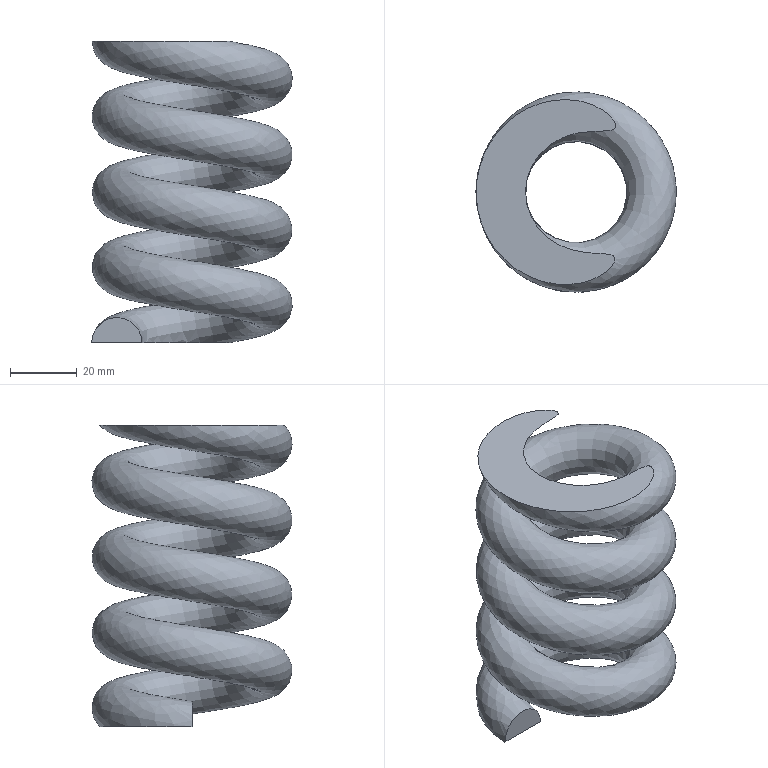Part | NX | features MAIN_BODY 2 | 1 solid | 4 faces | box 59.9 x 59.795 x 90 mm | volume 97193 mm3 | plane 3 | spline 1
STEP:
#1=CARTESIAN_POINT('',(-585.,25.,130.));
#2=VERTEX_POINT('',#1);
#3=CARTESIAN_POINT('',(-570.,25.,130.));
#4=VERTEX_POINT('',#3);
#5=CARTESIAN_POINT('',(-577.5,25.,130.));
#6=DIRECTION('',(0.,1.,0.));
#7=DIRECTION('',(0.,0.,-1.));
#8=AXIS2_PLACEMENT_3D('',#5,#6,#7);
#9=CIRCLE('',#8,7.5);
#10=EDGE_CURVE('',#2,#4,#9,.T.);
#11=ORIENTED_EDGE('',*,*,#10,.T.);
#12=CARTESIAN_POINT('',(-585.,25.,130.));
#13=CARTESIAN_POINT('',(-585.,27.045,130.));
#14=CARTESIAN_POINT('',(-584.488,31.04,130.));
#15=CARTESIAN_POINT('',(-581.859,38.786,130.));
#16=CARTESIAN_POINT('',(-576.924,45.368,130.));
#17=CARTESIAN_POINT('',(-570.139,49.94,130.));
#18=CARTESIAN_POINT('',(-564.47,52.09,130.));
#19=CARTESIAN_POINT('',(-559.395,52.727,130.));
#20=CARTESIAN_POINT('',(-555.366,52.475,130.));
#21=CARTESIAN_POINT('',(-552.35,51.874,130.));
#22=CARTESIAN_POINT('',(-549.498,50.852,130.));
#23=CARTESIAN_POINT('',(-547.249,49.607,130.));
#24=CARTESIAN_POINT('',(-545.63,48.346,130.));
#25=CARTESIAN_POINT('',(-544.556,47.258,130.));
#26=CARTESIAN_POINT('',(-543.829,46.178,130.));
#27=CARTESIAN_POINT('',(-543.527,45.186,130.));
#28=CARTESIAN_POINT('',(-543.63,44.385,130.));
#29=CARTESIAN_POINT('',(-544.226,43.836,130.));
#30=CARTESIAN_POINT('',(-545.199,43.494,130.));
#31=CARTESIAN_POINT('',(-546.469,43.349,130.));
#32=CARTESIAN_POINT('',(-548.002,43.281,130.));
#33=CARTESIAN_POINT('',(-550.045,43.207,130.));
#34=CARTESIAN_POINT('',(-552.6,43.018,130.));
#35=CARTESIAN_POINT('',(-555.61,42.46,130.));
#36=CARTESIAN_POINT('',(-558.514,41.525,130.));
#37=CARTESIAN_POINT('',(-562.2,39.726,130.));
#38=CARTESIAN_POINT('',(-566.15,36.439,130.));
#39=CARTESIAN_POINT('',(-569.39,31.132,130.));
#40=CARTESIAN_POINT('',(-570.,27.054,130.));
#41=CARTESIAN_POINT('',(-570.,25.,130.));
#42=B_SPLINE_CURVE_WITH_KNOTS('',3,(#12,#13,#14,#15,#16,#17,#18,#19,#20,#21,#22,#23,#24,#25,#26,#27,#28,#29,#30,#31,#32,#33,#34,#35,#36,#37,#38,#39,#40,#41),.UNSPECIFIED.,.F.,.F.,(4,1,1,1,1,1,1,1,1,1,1,1,1,1,1,1,1,1,1,1,1,1,1,1,1,1,1,4),(0.,0.006042,0.01208,0.02417,0.03021,0.03625,0.0423,0.04532,0.04834,0.05136,0.05438,0.05589,0.0574,0.05891,0.05967,0.06042,0.06118,0.06193,0.06345,0.06496,0.06647,0.06949,0.07251,0.07553,0.07855,0.08459,0.09064,0.09668),.UNSPECIFIED.);
#43=EDGE_CURVE('',#2,#4,#42,.T.);
#44=ORIENTED_EDGE('',*,*,#43,.F.);
#45=EDGE_LOOP('',(#11,#44));
#46=FACE_BOUND('',#45,.T.);
#47=CARTESIAN_POINT('',(-550.036,43.104,220.));
#48=VERTEX_POINT('',#47);
#49=CARTESIAN_POINT('',(-548.485,43.153,220.));
#50=CARTESIAN_POINT('',(-550.563,43.099,220.));
#51=CARTESIAN_POINT('',(-553.055,42.902,220.));
#52=CARTESIAN_POINT('',(-556.004,42.327,220.));
#53=CARTESIAN_POINT('',(-558.885,41.355,220.));
#54=CARTESIAN_POINT('',(-562.502,39.519,220.));
#55=CARTESIAN_POINT('',(-566.39,36.179,220.));
#56=CARTESIAN_POINT('',(-569.464,30.845,220.));
#57=CARTESIAN_POINT('',(-570.497,24.764,220.));
#58=CARTESIAN_POINT('',(-569.32,18.707,220.));
#59=CARTESIAN_POINT('',(-566.126,13.433,220.));
#60=CARTESIAN_POINT('',(-562.172,10.17,220.));
#61=CARTESIAN_POINT('',(-558.517,8.387,220.));
#62=CARTESIAN_POINT('',(-555.622,7.457,220.));
#63=CARTESIAN_POINT('',(-552.661,6.901,220.));
#64=CARTESIAN_POINT('',(-550.128,6.704,220.));
#65=CARTESIAN_POINT('',(-548.096,6.631,220.));
#66=CARTESIAN_POINT('',(-546.57,6.571,220.));
#67=CARTESIAN_POINT('',(-545.31,6.452,220.));
#68=CARTESIAN_POINT('',(-544.308,6.16,220.));
#69=CARTESIAN_POINT('',(-543.636,5.702,220.));
#70=CARTESIAN_POINT('',(-543.401,4.908,220.));
#71=CARTESIAN_POINT('',(-543.652,3.875,220.));
#72=CARTESIAN_POINT('',(-544.361,2.77,220.));
#73=CARTESIAN_POINT('',(-545.431,1.655,220.));
#74=CARTESIAN_POINT('',(-547.063,0.3637,220.));
#75=CARTESIAN_POINT('',(-549.293,-0.8896,220.));
#76=CARTESIAN_POINT('',(-552.223,-1.947,220.));
#77=CARTESIAN_POINT('',(-555.215,-2.548,220.));
#78=CARTESIAN_POINT('',(-559.345,-2.814,220.));
#79=CARTESIAN_POINT('',(-564.458,-2.164,220.));
#80=CARTESIAN_POINT('',(-570.219,0.05404,220.));
#81=CARTESIAN_POINT('',(-575.334,3.544,220.));
#82=CARTESIAN_POINT('',(-579.552,8.075,220.));
#83=CARTESIAN_POINT('',(-582.629,13.384,220.));
#84=CARTESIAN_POINT('',(-585.154,21.248,220.));
#85=CARTESIAN_POINT('',(-584.972,31.672,220.));
#86=CARTESIAN_POINT('',(-580.41,41.124,220.));
#87=CARTESIAN_POINT('',(-574.622,46.932,220.));
#88=CARTESIAN_POINT('',(-569.388,50.258,220.));
#89=CARTESIAN_POINT('',(-563.56,52.246,220.));
#90=CARTESIAN_POINT('',(-558.451,52.722,220.));
#91=CARTESIAN_POINT('',(-554.35,52.309,220.));
#92=CARTESIAN_POINT('',(-551.358,51.577,220.));
#93=CARTESIAN_POINT('',(-548.504,50.408,220.));
#94=CARTESIAN_POINT('',(-546.301,49.038,220.));
#95=CARTESIAN_POINT('',(-544.751,47.66,220.));
#96=CARTESIAN_POINT('',(-543.919,46.664,220.));
#97=CARTESIAN_POINT('',(-543.418,45.748,220.));
#98=CARTESIAN_POINT('',(-543.184,45.001,220.));
#99=CARTESIAN_POINT('',(-543.273,44.187,220.));
#100=CARTESIAN_POINT('',(-543.882,43.634,220.));
#101=CARTESIAN_POINT('',(-544.627,43.392,220.));
#102=CARTESIAN_POINT('',(-545.643,43.229,220.));
#103=CARTESIAN_POINT('',(-546.939,43.175,220.));
#104=CARTESIAN_POINT('',(-548.485,43.153,220.));
#105=CARTESIAN_POINT('',(-550.563,43.099,220.));
#106=CARTESIAN_POINT('',(-553.055,42.902,220.));
#107=B_SPLINE_CURVE_WITH_KNOTS('',3,(#49,#50,#51,#52,#53,#54,#55,#56,#57,#58,#59,#60,#61,#62,#63,#64,#65,#66,#67,#68,#69,#70,#71,#72,#73,#74,#75,#76,#77,#78,#79,#80,#81,#82,#83,#84,#85,#86,#87,#88,#89,#90,#91,#92,#93,#94,#95,#96,#97,#98,#99,#100,#101,#102,#103,#104,#105,#106),.UNSPECIFIED.,.T.,.F.,(1,1,1,1,1,1,1,1,1,1,1,1,1,1,1,1,1,1,1,1,1,1,1,1,1,1,1,1,1,1,1,1,1,1,1,1,1,1,1,1,1,1,1,1,1,1,1,1,1,1,1,1,1,1,1,1,1,1,1,1,1,1),(-0.004503,-0.003002,-0.001501,0.,0.003002,0.006004,0.009006,0.01201,0.01801,0.02401,0.03002,0.03602,0.04203,0.04803,0.05103,0.05403,0.05704,0.06004,0.06154,0.06304,0.06454,0.06529,0.06604,0.06679,0.06754,0.06904,0.07054,0.07204,0.07505,0.07805,0.08105,0.08405,0.09006,0.09606,0.1021,0.1081,0.1141,0.1201,0.1321,0.1441,0.1501,0.1561,0.1621,0.1681,0.1711,0.1741,0.1771,0.1801,0.1816,0.1831,0.1839,0.1846,0.1854,0.1861,0.1869,0.1876,0.1891,0.1906,0.1921,0.1951,0.1981,0.2011),.UNSPECIFIED.);
#108=EDGE_CURVE('',#48,#48,#107,.T.);
#109=ORIENTED_EDGE('',*,*,#108,.T.);
#110=EDGE_LOOP('',(#109));
#111=FACE_BOUND('',#110,.T.);
#112=CARTESIAN_POINT('',(-585.,25.,127.348));
#113=CARTESIAN_POINT('',(-585.,30.508,128.225));
#114=CARTESIAN_POINT('',(-581.873,41.672,130.003));
#115=CARTESIAN_POINT('',(-569.487,53.277,132.606));
#116=CARTESIAN_POINT('',(-552.814,56.781,135.219));
#117=CARTESIAN_POINT('',(-536.716,51.119,137.836));
#118=CARTESIAN_POINT('',(-525.89,37.929,140.453));
#119=CARTESIAN_POINT('',(-523.482,21.066,143.066));
#120=CARTESIAN_POINT('',(-530.147,5.463,145.668));
#121=CARTESIAN_POINT('',(-543.864,-4.371,148.256));
#122=CARTESIAN_POINT('',(-560.569,-5.646,150.825));
#123=CARTESIAN_POINT('',(-575.379,1.855,153.371));
#124=CARTESIAN_POINT('',(-584.048,15.804,155.89));
#125=CARTESIAN_POINT('',(-584.226,32.016,158.376));
#126=CARTESIAN_POINT('',(-576.083,45.772,160.828));
#127=CARTESIAN_POINT('',(-562.21,53.186,163.24));
#128=CARTESIAN_POINT('',(-546.781,52.344,165.61));
#129=CARTESIAN_POINT('',(-534.267,43.786,167.935));
#130=CARTESIAN_POINT('',(-528.143,30.264,170.211));
#131=CARTESIAN_POINT('',(-529.877,15.849,172.438));
#132=CARTESIAN_POINT('',(-538.633,4.698,174.612));
#133=CARTESIAN_POINT('',(-551.571,-0.1739,176.732));
#134=CARTESIAN_POINT('',(-564.808,2.311,178.797));
#135=CARTESIAN_POINT('',(-574.563,11.056,180.807));
#136=CARTESIAN_POINT('',(-578.261,23.244,182.76));
#137=CARTESIAN_POINT('',(-575.19,35.226,184.657));
#138=CARTESIAN_POINT('',(-566.609,43.62,186.498));
#139=CARTESIAN_POINT('',(-555.267,46.268,188.284));
#140=CARTESIAN_POINT('',(-544.533,42.752,190.016));
#141=CARTESIAN_POINT('',(-537.399,34.439,191.696));
#142=CARTESIAN_POINT('',(-535.67,23.953,193.326));
#143=CARTESIAN_POINT('',(-539.512,14.383,194.907));
#144=CARTESIAN_POINT('',(-547.526,8.372,196.444));
#145=CARTESIAN_POINT('',(-557.221,7.417,197.938));
#146=CARTESIAN_POINT('',(-565.775,11.52,199.393));
#147=CARTESIAN_POINT('',(-570.835,19.272,200.812));
#148=CARTESIAN_POINT('',(-571.129,28.317,202.2));
#149=CARTESIAN_POINT('',(-566.78,36.049,203.561));
#150=CARTESIAN_POINT('',(-559.181,40.323,204.898));
#151=CARTESIAN_POINT('',(-550.59,40.043,206.216));
#152=CARTESIAN_POINT('',(-543.47,35.396,207.52));
#153=CARTESIAN_POINT('',(-539.821,27.788,208.814));
#154=CARTESIAN_POINT('',(-540.645,19.422,210.103));
#155=CARTESIAN_POINT('',(-545.689,12.698,211.392));
#156=CARTESIAN_POINT('',(-553.516,9.556,212.686));
#157=CARTESIAN_POINT('',(-561.9,10.938,213.989));
#158=CARTESIAN_POINT('',(-568.416,16.531,215.306));
#159=CARTESIAN_POINT('',(-571.127,24.806,216.641));
#160=CARTESIAN_POINT('',(-569.113,33.433,218.));
#161=CARTESIAN_POINT('',(-562.795,39.892,219.385));
#162=CARTESIAN_POINT('',(-553.844,42.186,220.802));
#163=CARTESIAN_POINT('',(-547.329,40.209,221.847));
#164=CARTESIAN_POINT('',(-544.409,38.147,222.415));
#165=CARTESIAN_POINT('',(-544.024,37.85,222.493));
#166=CARTESIAN_POINT('',(-585.,25.,132.652));
#167=CARTESIAN_POINT('',(-585.,29.684,133.397));
#168=CARTESIAN_POINT('',(-581.906,40.732,135.157));
#169=CARTESIAN_POINT('',(-569.784,52.089,137.705));
#170=CARTESIAN_POINT('',(-553.698,55.469,140.225));
#171=CARTESIAN_POINT('',(-538.388,50.085,142.714));
#172=CARTESIAN_POINT('',(-528.237,37.717,145.168));
#173=CARTESIAN_POINT('',(-526.011,22.125,147.583));
#174=CARTESIAN_POINT('',(-532.088,7.896,149.956));
#175=CARTESIAN_POINT('',(-544.427,-0.9495,152.285));
#176=CARTESIAN_POINT('',(-559.252,-2.08,154.565));
#177=CARTESIAN_POINT('',(-572.225,4.49,156.795));
#178=CARTESIAN_POINT('',(-579.722,16.553,158.973));
#179=CARTESIAN_POINT('',(-579.874,30.402,161.097));
#180=CARTESIAN_POINT('',(-573.001,42.013,163.166));
#181=CARTESIAN_POINT('',(-561.422,48.201,165.18));
#182=CARTESIAN_POINT('',(-548.68,47.506,167.137));
#183=CARTESIAN_POINT('',(-538.447,40.508,169.038));
#184=CARTESIAN_POINT('',(-533.484,29.549,170.883));
#185=CARTESIAN_POINT('',(-534.878,17.961,172.673));
#186=CARTESIAN_POINT('',(-541.87,9.057,174.409));
#187=CARTESIAN_POINT('',(-552.143,5.189,176.092));
#188=CARTESIAN_POINT('',(-562.61,7.154,177.726));
#189=CARTESIAN_POINT('',(-570.305,14.052,179.311));
#190=CARTESIAN_POINT('',(-573.22,23.658,180.85));
#191=CARTESIAN_POINT('',(-570.796,33.114,182.347));
#192=CARTESIAN_POINT('',(-564.002,39.76,183.805));
#193=CARTESIAN_POINT('',(-554.972,41.868,185.227));
#194=CARTESIAN_POINT('',(-546.358,39.046,186.617));
#195=CARTESIAN_POINT('',(-540.573,32.306,187.979));
#196=CARTESIAN_POINT('',(-539.153,23.693,189.318));
#197=CARTESIAN_POINT('',(-542.358,15.71,190.637));
#198=CARTESIAN_POINT('',(-549.164,10.604,191.942));
#199=CARTESIAN_POINT('',(-557.565,9.777,193.236));
#200=CARTESIAN_POINT('',(-565.146,13.413,194.526));
#201=CARTESIAN_POINT('',(-569.739,20.452,195.815));
#202=CARTESIAN_POINT('',(-570.014,28.879,197.108));
#203=CARTESIAN_POINT('',(-565.851,36.28,198.41));
#204=CARTESIAN_POINT('',(-558.373,40.486,199.726));
#205=CARTESIAN_POINT('',(-549.679,40.203,201.06));
#206=CARTESIAN_POINT('',(-542.271,35.367,202.416));
#207=CARTESIAN_POINT('',(-538.369,27.233,203.8));
#208=CARTESIAN_POINT('',(-539.273,18.053,205.215));
#209=CARTESIAN_POINT('',(-544.945,10.492,206.664));
#210=CARTESIAN_POINT('',(-553.949,6.878,208.152));
#211=CARTESIAN_POINT('',(-563.793,8.5,209.682));
#212=CARTESIAN_POINT('',(-571.586,15.188,211.257));
#213=CARTESIAN_POINT('',(-574.879,25.242,212.879));
#214=CARTESIAN_POINT('',(-572.4,35.863,214.552));
#215=CARTESIAN_POINT('',(-564.538,43.899,216.276));
#216=CARTESIAN_POINT('',(-553.306,46.778,218.054));
#217=CARTESIAN_POINT('',(-545.083,44.283,219.372));
#218=CARTESIAN_POINT('',(-541.39,41.674,220.092));
#219=CARTESIAN_POINT('',(-540.904,41.298,220.189));
#220=CARTESIAN_POINT('',(-583.674,25.,136.174));
#221=CARTESIAN_POINT('',(-583.674,28.959,136.804));
#222=CARTESIAN_POINT('',(-580.747,39.411,138.469));
#223=CARTESIAN_POINT('',(-569.324,50.113,140.87));
#224=CARTESIAN_POINT('',(-554.321,53.267,143.221));
#225=CARTESIAN_POINT('',(-540.187,48.296,145.519));
#226=CARTESIAN_POINT('',(-530.909,36.992,147.762));
#227=CARTESIAN_POINT('',(-528.895,22.884,149.947));
#228=CARTESIAN_POINT('',(-534.34,10.136,152.073));
#229=CARTESIAN_POINT('',(-545.29,2.285,154.139));
#230=CARTESIAN_POINT('',(-558.325,1.291,156.144));
#231=CARTESIAN_POINT('',(-569.63,7.017,158.087));
#232=CARTESIAN_POINT('',(-576.109,17.441,159.969));
#233=CARTESIAN_POINT('',(-576.239,29.314,161.791));
#234=CARTESIAN_POINT('',(-570.389,39.196,163.552));
#235=CARTESIAN_POINT('',(-560.598,44.429,165.254));
#236=CARTESIAN_POINT('',(-549.882,43.844,166.9));
#237=CARTESIAN_POINT('',(-541.317,37.986,168.491));
#238=CARTESIAN_POINT('',(-537.176,28.844,170.031));
#239=CARTESIAN_POINT('',(-538.337,19.195,171.521));
#240=CARTESIAN_POINT('',(-544.155,11.786,172.966));
#241=CARTESIAN_POINT('',(-552.714,8.563,174.368));
#242=CARTESIAN_POINT('',(-561.459,10.205,175.733));
#243=CARTESIAN_POINT('',(-567.919,15.996,177.063));
#244=CARTESIAN_POINT('',(-570.383,24.116,178.365));
#245=CARTESIAN_POINT('',(-568.316,32.179,179.641));
#246=CARTESIAN_POINT('',(-562.459,37.91,180.898));
#247=CARTESIAN_POINT('',(-554.572,39.751,182.14));
#248=CARTESIAN_POINT('',(-546.937,37.249,183.372));
#249=CARTESIAN_POINT('',(-541.724,31.175,184.6));
#250=CARTESIAN_POINT('',(-540.422,23.273,185.828));
#251=CARTESIAN_POINT('',(-543.419,15.806,187.062));
#252=CARTESIAN_POINT('',(-549.913,10.934,188.307));
#253=CARTESIAN_POINT('',(-558.096,10.129,189.568));
#254=CARTESIAN_POINT('',(-565.634,13.744,190.85));
#255=CARTESIAN_POINT('',(-570.296,20.887,192.158));
#256=CARTESIAN_POINT('',(-570.58,29.609,193.496));
#257=CARTESIAN_POINT('',(-566.189,37.415,194.87));
#258=CARTESIAN_POINT('',(-558.162,41.93,196.282));
#259=CARTESIAN_POINT('',(-548.677,41.621,197.738));
#260=CARTESIAN_POINT('',(-540.476,36.269,199.239));
#261=CARTESIAN_POINT('',(-536.101,27.147,200.791));
#262=CARTESIAN_POINT('',(-537.125,16.736,202.395));
#263=CARTESIAN_POINT('',(-543.619,8.08,204.055));
#264=CARTESIAN_POINT('',(-554.005,3.911,205.771));
#265=CARTESIAN_POINT('',(-565.43,5.795,207.547));
#266=CARTESIAN_POINT('',(-574.514,13.591,209.383));
#267=CARTESIAN_POINT('',(-578.364,25.345,211.28));
#268=CARTESIAN_POINT('',(-575.461,37.781,213.238));
#269=CARTESIAN_POINT('',(-566.253,47.194,215.258));
#270=CARTESIAN_POINT('',(-553.109,50.563,217.338));
#271=CARTESIAN_POINT('',(-543.506,47.649,218.877));
#272=CARTESIAN_POINT('',(-539.199,44.608,219.716));
#273=CARTESIAN_POINT('',(-538.632,44.17,219.83));
#274=CARTESIAN_POINT('',(-580.152,25.,137.5));
#275=CARTESIAN_POINT('',(-580.152,28.281,138.022));
#276=CARTESIAN_POINT('',(-577.618,37.327,139.463));
#277=CARTESIAN_POINT('',(-567.652,46.665,141.558));
#278=CARTESIAN_POINT('',(-554.635,49.4,143.597));
#279=CARTESIAN_POINT('',(-542.431,45.108,145.582));
#280=CARTESIAN_POINT('',(-534.453,35.389,147.51));
#281=CARTESIAN_POINT('',(-532.727,23.298,149.383));
#282=CARTESIAN_POINT('',(-537.383,12.399,151.201));
#283=CARTESIAN_POINT('',(-546.731,5.697,152.965));
#284=CARTESIAN_POINT('',(-557.856,4.848,154.676));
#285=CARTESIAN_POINT('',(-567.514,9.74,156.336));
#286=CARTESIAN_POINT('',(-573.06,18.665,157.947));
#287=CARTESIAN_POINT('',(-573.172,28.868,159.512));
#288=CARTESIAN_POINT('',(-568.119,37.405,161.034));
#289=CARTESIAN_POINT('',(-559.602,41.956,162.515));
#290=CARTESIAN_POINT('',(-550.203,41.443,163.958));
#291=CARTESIAN_POINT('',(-542.611,36.251,165.369));
#292=CARTESIAN_POINT('',(-538.897,28.05,166.749));
#293=CARTESIAN_POINT('',(-539.952,19.275,168.105));
#294=CARTESIAN_POINT('',(-545.326,12.433,169.439));
#295=CARTESIAN_POINT('',(-553.365,9.406,170.756));
#296=CARTESIAN_POINT('',(-561.73,10.976,172.062));
#297=CARTESIAN_POINT('',(-568.031,16.625,173.359));
#298=CARTESIAN_POINT('',(-570.483,24.705,174.654));
#299=CARTESIAN_POINT('',(-568.383,32.897,175.951));
#300=CARTESIAN_POINT('',(-562.307,38.84,177.255));
#301=CARTESIAN_POINT('',(-553.958,40.789,178.57));
#302=CARTESIAN_POINT('',(-545.712,38.088,179.9));
#303=CARTESIAN_POINT('',(-539.975,31.403,181.251));
#304=CARTESIAN_POINT('',(-538.515,22.551,182.627));
#305=CARTESIAN_POINT('',(-541.927,14.053,184.032));
#306=CARTESIAN_POINT('',(-549.424,8.429,185.469));
#307=CARTESIAN_POINT('',(-558.987,7.488,186.943));
#308=CARTESIAN_POINT('',(-567.885,11.756,188.456));
#309=CARTESIAN_POINT('',(-573.433,20.256,190.013));
#310=CARTESIAN_POINT('',(-573.773,30.699,191.615));
#311=CARTESIAN_POINT('',(-568.495,40.082,193.266));
#312=CARTESIAN_POINT('',(-558.825,45.521,194.967));
#313=CARTESIAN_POINT('',(-547.395,45.149,196.721));
#314=CARTESIAN_POINT('',(-537.524,38.706,198.529));
#315=CARTESIAN_POINT('',(-532.272,27.757,200.391));
#316=CARTESIAN_POINT('',(-533.498,15.311,202.309));
#317=CARTESIAN_POINT('',(-541.221,5.015,204.283));
#318=CARTESIAN_POINT('',(-553.5,0.08651,206.312));
#319=CARTESIAN_POINT('',(-566.912,2.298,208.397));
#320=CARTESIAN_POINT('',(-577.493,11.379,210.535));
#321=CARTESIAN_POINT('',(-581.941,24.958,212.727));
#322=CARTESIAN_POINT('',(-578.617,39.198,214.969));
#323=CARTESIAN_POINT('',(-568.17,49.877,217.26));
#324=CARTESIAN_POINT('',(-553.402,53.663,219.598));
#325=CARTESIAN_POINT('',(-542.717,50.421,221.311));
#326=CARTESIAN_POINT('',(-537.949,47.064,222.238));
#327=CARTESIAN_POINT('',(-537.322,46.581,222.364));
#328=CARTESIAN_POINT('',(-574.848,25.,137.5));
#329=CARTESIAN_POINT('',(-574.848,27.57,137.909));
#330=CARTESIAN_POINT('',(-572.895,34.543,139.02));
#331=CARTESIAN_POINT('',(-565.023,41.919,140.674));
#332=CARTESIAN_POINT('',(-554.774,44.073,142.28));
#333=CARTESIAN_POINT('',(-545.18,40.699,143.84));
#334=CARTESIAN_POINT('',(-538.906,33.055,145.357));
#335=CARTESIAN_POINT('',(-537.545,23.523,146.833));
#336=CARTESIAN_POINT('',(-541.232,14.89,148.273));
#337=CARTESIAN_POINT('',(-548.688,9.545,149.68));
#338=CARTESIAN_POINT('',(-557.645,8.862,151.058));
#339=CARTESIAN_POINT('',(-565.514,12.847,152.41));
#340=CARTESIAN_POINT('',(-570.099,20.225,153.742));
#341=CARTESIAN_POINT('',(-570.193,28.804,155.058));
#342=CARTESIAN_POINT('',(-565.861,36.122,156.362));
#343=CARTESIAN_POINT('',(-558.401,40.109,157.659));
#344=CARTESIAN_POINT('',(-549.97,39.649,158.954));
#345=CARTESIAN_POINT('',(-542.987,34.873,160.252));
#346=CARTESIAN_POINT('',(-539.477,27.124,161.556));
#347=CARTESIAN_POINT('',(-540.502,18.601,162.873));
#348=CARTESIAN_POINT('',(-545.87,11.766,164.206));
#349=CARTESIAN_POINT('',(-554.13,8.655,165.559));
#350=CARTESIAN_POINT('',(-562.966,10.314,166.938));
#351=CARTESIAN_POINT('',(-569.802,16.443,168.346));
#352=CARTESIAN_POINT('',(-572.531,25.435,169.787));
#353=CARTESIAN_POINT('',(-570.138,34.772,171.265));
#354=CARTESIAN_POINT('',(-563.061,41.694,172.784));
#355=CARTESIAN_POINT('',(-553.144,44.009,174.345));
#356=CARTESIAN_POINT('',(-543.181,40.745,175.953));
#357=CARTESIAN_POINT('',(-536.146,32.548,177.61));
#358=CARTESIAN_POINT('',(-534.335,21.563,179.317));
#359=CARTESIAN_POINT('',(-538.609,10.914,181.077));
#360=CARTESIAN_POINT('',(-548.071,3.817,182.891));
#361=CARTESIAN_POINT('',(-560.197,2.623,184.76));
#362=CARTESIAN_POINT('',(-571.51,8.049,186.684));
#363=CARTESIAN_POINT('',(-578.568,18.862,188.664));
#364=CARTESIAN_POINT('',(-579.,32.128,190.7));
#365=CARTESIAN_POINT('',(-572.316,44.01,192.79));
#366=CARTESIAN_POINT('',(-560.127,50.866,194.935));
#367=CARTESIAN_POINT('',(-545.808,50.4,197.132));
#368=CARTESIAN_POINT('',(-533.532,42.387,199.38));
#369=CARTESIAN_POINT('',(-527.055,28.885,201.677));
#370=CARTESIAN_POINT('',(-528.552,13.68,204.02));
#371=CARTESIAN_POINT('',(-537.891,1.231,206.407));
#372=CARTESIAN_POINT('',(-552.575,-4.663,208.833));
#373=CARTESIAN_POINT('',(-568.429,-2.05,211.297));
#374=CARTESIAN_POINT('',(-580.785,8.555,213.795));
#375=CARTESIAN_POINT('',(-585.914,24.212,216.321));
#376=CARTESIAN_POINT('',(-582.131,40.418,218.873));
#377=CARTESIAN_POINT('',(-570.401,52.408,221.446));
#378=CARTESIAN_POINT('',(-554.044,56.601,224.035));
#379=CARTESIAN_POINT('',(-542.374,53.06,225.906));
#380=CARTESIAN_POINT('',(-537.203,49.434,226.91));
#381=CARTESIAN_POINT('',(-536.523,48.912,227.047));
#382=CARTESIAN_POINT('',(-571.326,25.,136.174));
#383=CARTESIAN_POINT('',(-571.326,27.304,136.541));
#384=CARTESIAN_POINT('',(-569.75,32.929,137.437));
#385=CARTESIAN_POINT('',(-563.202,39.064,138.813));
#386=CARTESIAN_POINT('',(-554.645,40.862,140.154));
#387=CARTESIAN_POINT('',(-546.587,38.028,141.464));
#388=CARTESIAN_POINT('',(-541.276,31.558,142.748));
#389=CARTESIAN_POINT('',(-540.113,23.408,144.01));
#390=CARTESIAN_POINT('',(-543.304,15.937,145.256));
#391=CARTESIAN_POINT('',(-549.847,11.246,146.491));
#392=CARTESIAN_POINT('',(-557.834,10.636,147.719));
#393=CARTESIAN_POINT('',(-564.974,14.253,148.947));
#394=CARTESIAN_POINT('',(-569.213,21.074,150.178));
#395=CARTESIAN_POINT('',(-569.302,29.165,151.419));
#396=CARTESIAN_POINT('',(-565.132,36.21,152.675));
#397=CARTESIAN_POINT('',(-557.8,40.128,153.95));
#398=CARTESIAN_POINT('',(-549.341,39.666,155.249));
#399=CARTESIAN_POINT('',(-542.191,34.777,156.577));
#400=CARTESIAN_POINT('',(-538.527,26.688,157.939));
#401=CARTESIAN_POINT('',(-539.617,17.626,159.339));
#402=CARTESIAN_POINT('',(-545.423,10.233,160.78));
#403=CARTESIAN_POINT('',(-554.495,6.817,162.267));
#404=CARTESIAN_POINT('',(-564.337,8.664,163.803));
#405=CARTESIAN_POINT('',(-572.043,15.573,165.39));
#406=CARTESIAN_POINT('',(-575.152,25.817,167.032));
#407=CARTESIAN_POINT('',(-572.402,36.545,168.73));
#408=CARTESIAN_POINT('',(-564.214,44.555,170.487));
#409=CARTESIAN_POINT('',(-552.677,47.248,172.304));
#410=CARTESIAN_POINT('',(-541.043,43.437,174.181));
#411=CARTESIAN_POINT('',(-532.809,33.843,176.12));
#412=CARTESIAN_POINT('',(-530.687,20.971,178.121));
#413=CARTESIAN_POINT('',(-535.694,8.498,180.182));
#414=CARTESIAN_POINT('',(-546.763,0.1949,182.304));
#415=CARTESIAN_POINT('',(-560.916,-1.198,184.485));
#416=CARTESIAN_POINT('',(-574.076,5.114,186.724));
#417=CARTESIAN_POINT('',(-582.252,17.642,189.018));
#418=CARTESIAN_POINT('',(-582.751,32.936,191.365));
#419=CARTESIAN_POINT('',(-575.086,46.562,193.762));
#420=CARTESIAN_POINT('',(-561.194,54.376,196.206));
#421=CARTESIAN_POINT('',(-544.982,53.848,198.694));
#422=CARTESIAN_POINT('',(-531.18,44.84,201.221));
#423=CARTESIAN_POINT('',(-523.953,29.773,203.784));
#424=CARTESIAN_POINT('',(-525.61,12.939,206.378));
#425=CARTESIAN_POINT('',(-535.865,-0.7312,208.999));
#426=CARTESIAN_POINT('',(-551.853,-7.149,211.641));
#427=CARTESIAN_POINT('',(-568.964,-4.328,214.301));
#428=CARTESIAN_POINT('',(-582.18,7.015,216.972));
#429=CARTESIAN_POINT('',(-587.615,23.607,219.649));
#430=CARTESIAN_POINT('',(-583.644,40.62,222.328));
#431=CARTESIAN_POINT('',(-571.448,53.087,225.003));
#432=CARTESIAN_POINT('',(-554.606,57.404,227.669));
#433=CARTESIAN_POINT('',(-542.708,53.794,229.576));
#434=CARTESIAN_POINT('',(-537.462,50.126,230.595));
#435=CARTESIAN_POINT('',(-536.773,49.599,230.733));
#436=CARTESIAN_POINT('',(-570.,25.,132.652));
#437=CARTESIAN_POINT('',(-570.,27.673,133.077));
#438=CARTESIAN_POINT('',(-568.548,32.858,133.903));
#439=CARTESIAN_POINT('',(-562.348,38.667,135.206));
#440=CARTESIAN_POINT('',(-554.092,40.402,136.5));
#441=CARTESIAN_POINT('',(-546.164,37.613,137.789));
#442=CARTESIAN_POINT('',(-540.83,31.115,139.078));
#443=CARTESIAN_POINT('',(-539.638,22.761,140.372));
#444=CARTESIAN_POINT('',(-542.977,14.943,141.676));
#445=CARTESIAN_POINT('',(-549.963,9.935,142.994));
#446=CARTESIAN_POINT('',(-558.656,9.272,144.331));
#447=CARTESIAN_POINT('',(-566.569,13.28,145.691));
#448=CARTESIAN_POINT('',(-571.346,20.967,147.079));
#449=CARTESIAN_POINT('',(-571.448,30.221,148.499));
#450=CARTESIAN_POINT('',(-566.615,38.386,149.954));
#451=CARTESIAN_POINT('',(-558.024,42.977,151.448));
#452=CARTESIAN_POINT('',(-548.022,42.431,152.984));
#453=CARTESIAN_POINT('',(-539.509,36.609,154.565));
#454=CARTESIAN_POINT('',(-535.125,26.93,156.195));
#455=CARTESIAN_POINT('',(-536.433,16.054,157.875));
#456=CARTESIAN_POINT('',(-543.409,7.171,159.607));
#457=CARTESIAN_POINT('',(-554.307,3.067,161.393));
#458=CARTESIAN_POINT('',(-566.106,5.282,163.234));
#459=CARTESIAN_POINT('',(-575.315,13.538,165.131));
#460=CARTESIAN_POINT('',(-579.013,25.724,167.084));
#461=CARTESIAN_POINT('',(-575.759,38.417,169.093));
#462=CARTESIAN_POINT('',(-566.134,47.832,171.158));
#463=CARTESIAN_POINT('',(-552.67,50.976,173.278));
#464=CARTESIAN_POINT('',(-539.198,46.562,175.452));
#465=CARTESIAN_POINT('',(-529.743,35.546,177.679));
#466=CARTESIAN_POINT('',(-527.328,20.897,179.955));
#467=CARTESIAN_POINT('',(-532.974,6.832,182.28));
#468=CARTESIAN_POINT('',(-545.337,-2.441,184.65));
#469=CARTESIAN_POINT('',(-560.99,-3.982,187.062));
#470=CARTESIAN_POINT('',(-575.4,2.929,189.513));
#471=CARTESIAN_POINT('',(-584.264,16.51,192.));
#472=CARTESIAN_POINT('',(-584.798,32.92,194.518));
#473=CARTESIAN_POINT('',(-576.659,47.39,197.064));
#474=CARTESIAN_POINT('',(-562.056,55.604,199.633));
#475=CARTESIAN_POINT('',(-545.191,55.055,202.221));
#476=CARTESIAN_POINT('',(-530.979,45.779,204.824));
#477=CARTESIAN_POINT('',(-523.614,30.423,207.436));
#478=CARTESIAN_POINT('',(-525.285,13.441,210.053));
#479=CARTESIAN_POINT('',(-535.527,-0.2119,212.67));
#480=CARTESIAN_POINT('',(-551.334,-6.557,215.283));
#481=CARTESIAN_POINT('',(-568.085,-3.796,217.886));
#482=CARTESIAN_POINT('',(-580.898,7.201,220.476));
#483=CARTESIAN_POINT('',(-586.116,23.131,223.046));
#484=CARTESIAN_POINT('',(-582.339,39.311,225.594));
#485=CARTESIAN_POINT('',(-570.848,51.058,228.115));
#486=CARTESIAN_POINT('',(-555.124,55.088,230.604));
#487=CARTESIAN_POINT('',(-544.114,51.748,232.368));
#488=CARTESIAN_POINT('',(-539.28,48.376,233.306));
#489=CARTESIAN_POINT('',(-538.646,47.892,233.433));
#490=CARTESIAN_POINT('',(-570.,25.,127.348));
#491=CARTESIAN_POINT('',(-570.,28.497,127.905));
#492=CARTESIAN_POINT('',(-568.515,33.798,128.749));
#493=CARTESIAN_POINT('',(-562.051,39.854,130.108));
#494=CARTESIAN_POINT('',(-553.208,41.713,131.494));
#495=CARTESIAN_POINT('',(-544.491,38.647,132.911));
#496=CARTESIAN_POINT('',(-538.483,31.328,134.363));
#497=CARTESIAN_POINT('',(-537.109,21.702,135.854));
#498=CARTESIAN_POINT('',(-541.036,12.51,137.387));
#499=CARTESIAN_POINT('',(-549.4,6.513,138.965));
#500=CARTESIAN_POINT('',(-559.972,5.707,140.591));
#501=CARTESIAN_POINT('',(-569.723,10.645,142.268));
#502=CARTESIAN_POINT('',(-575.672,20.218,143.996));
#503=CARTESIAN_POINT('',(-575.799,31.836,145.778));
#504=CARTESIAN_POINT('',(-569.697,42.144,147.615));
#505=CARTESIAN_POINT('',(-558.812,47.961,149.508));
#506=CARTESIAN_POINT('',(-546.123,47.269,151.457));
#507=CARTESIAN_POINT('',(-535.329,39.887,153.462));
#508=CARTESIAN_POINT('',(-529.784,27.644,155.523));
#509=CARTESIAN_POINT('',(-531.433,13.942,157.64));
#510=CARTESIAN_POINT('',(-540.173,2.812,159.81));
#511=CARTESIAN_POINT('',(-553.735,-2.295,162.032));
#512=CARTESIAN_POINT('',(-568.304,0.4398,164.306));
#513=CARTESIAN_POINT('',(-579.573,10.542,166.627));
#514=CARTESIAN_POINT('',(-584.054,25.31,168.994));
#515=CARTESIAN_POINT('',(-580.153,40.529,171.403));
#516=CARTESIAN_POINT('',(-568.742,51.693,173.851));
#517=CARTESIAN_POINT('',(-552.965,55.376,176.336));
#518=CARTESIAN_POINT('',(-537.373,50.268,178.852));
#519=CARTESIAN_POINT('',(-526.569,37.679,181.396));
#520=CARTESIAN_POINT('',(-523.845,21.158,183.964));
#521=CARTESIAN_POINT('',(-530.128,5.506,186.55));
#522=CARTESIAN_POINT('',(-543.699,-4.674,189.152));
#523=CARTESIAN_POINT('',(-560.646,-6.342,191.764));
#524=CARTESIAN_POINT('',(-576.03,1.036,194.38));
#525=CARTESIAN_POINT('',(-585.359,15.33,196.998));
#526=CARTESIAN_POINT('',(-585.913,32.358,199.611));
#527=CARTESIAN_POINT('',(-577.588,47.159,202.215));
#528=CARTESIAN_POINT('',(-562.864,55.441,204.806));
#529=CARTESIAN_POINT('',(-546.102,54.895,207.378));
#530=CARTESIAN_POINT('',(-532.178,45.808,209.927));
#531=CARTESIAN_POINT('',(-525.066,30.978,212.45));
#532=CARTESIAN_POINT('',(-526.657,14.81,214.942));
#533=CARTESIAN_POINT('',(-536.27,1.994,217.398));
#534=CARTESIAN_POINT('',(-550.902,-3.879,219.816));
#535=CARTESIAN_POINT('',(-566.192,-1.358,222.193));
#536=CARTESIAN_POINT('',(-577.728,8.543,224.524));
#537=CARTESIAN_POINT('',(-582.364,22.695,226.808));
#538=CARTESIAN_POINT('',(-579.053,36.881,229.042));
#539=CARTESIAN_POINT('',(-569.105,47.05,231.224));
#540=CARTESIAN_POINT('',(-555.662,50.496,233.352));
#541=CARTESIAN_POINT('',(-546.36,47.673,234.843));
#542=CARTESIAN_POINT('',(-542.298,44.85,235.63));
#543=CARTESIAN_POINT('',(-541.766,44.445,235.736));
#544=CARTESIAN_POINT('',(-571.326,25.,123.826));
#545=CARTESIAN_POINT('',(-571.326,29.222,124.498));
#546=CARTESIAN_POINT('',(-569.674,35.118,125.437));
#547=CARTESIAN_POINT('',(-562.511,41.83,126.942));
#548=CARTESIAN_POINT('',(-552.585,43.916,128.498));
#549=CARTESIAN_POINT('',(-542.693,40.437,130.106));
#550=CARTESIAN_POINT('',(-535.811,32.052,131.77));
#551=CARTESIAN_POINT('',(-534.225,20.943,133.491));
#552=CARTESIAN_POINT('',(-538.784,10.271,135.271));
#553=CARTESIAN_POINT('',(-548.537,3.278,137.111));
#554=CARTESIAN_POINT('',(-560.899,2.335,139.012));
#555=CARTESIAN_POINT('',(-572.317,8.118,140.975));
#556=CARTESIAN_POINT('',(-579.285,19.33,142.999));
#557=CARTESIAN_POINT('',(-579.434,32.924,145.084));
#558=CARTESIAN_POINT('',(-572.309,44.961,147.229));
#559=CARTESIAN_POINT('',(-559.636,51.734,149.433));
#560=CARTESIAN_POINT('',(-544.92,50.93,151.694));
#561=CARTESIAN_POINT('',(-532.459,42.408,154.009));
#562=CARTESIAN_POINT('',(-526.092,28.35,156.375));
#563=CARTESIAN_POINT('',(-527.974,12.708,158.791));
#564=CARTESIAN_POINT('',(-537.888,0.083,161.253));
#565=CARTESIAN_POINT('',(-553.165,-5.67,163.757));
#566=CARTESIAN_POINT('',(-569.455,-2.611,166.298));
#567=CARTESIAN_POINT('',(-581.959,8.598,168.874));
#568=CARTESIAN_POINT('',(-586.891,24.852,171.479));
#569=CARTESIAN_POINT('',(-582.633,41.464,174.109));
#570=CARTESIAN_POINT('',(-570.285,53.543,176.758));
#571=CARTESIAN_POINT('',(-553.365,57.493,179.423));
#572=CARTESIAN_POINT('',(-536.794,52.064,182.097));
#573=CARTESIAN_POINT('',(-525.418,38.81,184.775));
#574=CARTESIAN_POINT('',(-522.577,21.578,187.454));
#575=CARTESIAN_POINT('',(-529.067,5.409,190.126));
#576=CARTESIAN_POINT('',(-542.95,-5.004,192.787));
#577=CARTESIAN_POINT('',(-560.115,-6.694,195.432));
#578=CARTESIAN_POINT('',(-575.541,0.705,198.056));
#579=CARTESIAN_POINT('',(-584.802,14.895,200.655));
#580=CARTESIAN_POINT('',(-585.347,31.628,203.222));
#581=CARTESIAN_POINT('',(-577.249,46.024,205.755));
#582=CARTESIAN_POINT('',(-563.075,53.997,208.249));
#583=CARTESIAN_POINT('',(-547.104,53.477,210.7));
#584=CARTESIAN_POINT('',(-533.973,44.907,213.104));
#585=CARTESIAN_POINT('',(-527.334,31.064,215.459));
#586=CARTESIAN_POINT('',(-528.805,16.126,217.761));
#587=CARTESIAN_POINT('',(-537.597,4.406,220.008));
#588=CARTESIAN_POINT('',(-550.845,-0.9122,222.197));
#589=CARTESIAN_POINT('',(-564.555,1.348,224.328));
#590=CARTESIAN_POINT('',(-574.8,10.141,226.399));
#591=CARTESIAN_POINT('',(-578.879,22.592,228.408));
#592=CARTESIAN_POINT('',(-575.991,34.963,230.356));
#593=CARTESIAN_POINT('',(-567.39,43.755,232.242));
#594=CARTESIAN_POINT('',(-555.858,46.711,234.068));
#595=CARTESIAN_POINT('',(-547.938,44.307,235.337));
#596=CARTESIAN_POINT('',(-544.49,41.915,236.005));
#597=CARTESIAN_POINT('',(-544.038,41.572,236.096));
#598=CARTESIAN_POINT('',(-574.848,25.,122.5));
#599=CARTESIAN_POINT('',(-574.848,29.9,123.28));
#600=CARTESIAN_POINT('',(-572.803,37.203,124.443));
#601=CARTESIAN_POINT('',(-564.183,45.279,126.255));
#602=CARTESIAN_POINT('',(-552.271,47.782,128.121));
#603=CARTESIAN_POINT('',(-540.449,43.624,130.043));
#604=CARTESIAN_POINT('',(-532.267,33.656,132.021));
#605=CARTESIAN_POINT('',(-530.393,20.529,134.055));
#606=CARTESIAN_POINT('',(-535.741,8.007,136.143));
#607=CARTESIAN_POINT('',(-547.096,-0.1334,138.285));
#608=CARTESIAN_POINT('',(-561.368,-1.222,140.481));
#609=CARTESIAN_POINT('',(-574.434,5.395,142.727));
#610=CARTESIAN_POINT('',(-582.333,18.106,145.022));
#611=CARTESIAN_POINT('',(-582.501,33.37,147.363));
#612=CARTESIAN_POINT('',(-574.579,46.753,149.748));
#613=CARTESIAN_POINT('',(-560.631,54.207,152.173));
#614=CARTESIAN_POINT('',(-544.6,53.332,154.635));
#615=CARTESIAN_POINT('',(-531.165,44.143,157.131));
#616=CARTESIAN_POINT('',(-524.371,29.144,159.657));
#617=CARTESIAN_POINT('',(-526.358,12.628,162.208));
#618=CARTESIAN_POINT('',(-536.717,-0.5639,164.78));
#619=CARTESIAN_POINT('',(-552.513,-6.512,167.369));
#620=CARTESIAN_POINT('',(-569.184,-3.382,169.97));
#621=CARTESIAN_POINT('',(-581.847,7.97,172.578));
#622=CARTESIAN_POINT('',(-586.791,24.263,175.189));
#623=CARTESIAN_POINT('',(-582.566,40.746,177.799));
#624=CARTESIAN_POINT('',(-570.436,52.612,180.401));
#625=CARTESIAN_POINT('',(-553.979,56.454,182.993));
#626=CARTESIAN_POINT('',(-538.019,51.226,185.568));
#627=CARTESIAN_POINT('',(-527.168,38.582,188.124));
#628=CARTESIAN_POINT('',(-524.483,22.299,190.654));
#629=CARTESIAN_POINT('',(-530.559,7.162,193.156));
#630=CARTESIAN_POINT('',(-543.439,-2.499,195.625));
#631=CARTESIAN_POINT('',(-559.224,-4.053,198.058));
#632=CARTESIAN_POINT('',(-573.291,2.694,200.45));
#633=CARTESIAN_POINT('',(-581.665,15.525,202.8));
#634=CARTESIAN_POINT('',(-582.154,30.538,205.104));
#635=CARTESIAN_POINT('',(-574.944,43.357,207.359));
#636=CARTESIAN_POINT('',(-562.412,50.406,209.564));
#637=CARTESIAN_POINT('',(-548.386,49.949,211.716));
#638=CARTESIAN_POINT('',(-536.925,42.469,213.815));
#639=CARTESIAN_POINT('',(-531.162,30.454,215.859));
#640=CARTESIAN_POINT('',(-532.433,17.552,217.847));
#641=CARTESIAN_POINT('',(-539.995,7.471,219.779));
#642=CARTESIAN_POINT('',(-551.351,2.912,221.656));
#643=CARTESIAN_POINT('',(-563.074,4.845,223.478));
#644=CARTESIAN_POINT('',(-571.821,12.352,225.246));
#645=CARTESIAN_POINT('',(-575.302,22.979,226.961));
#646=CARTESIAN_POINT('',(-572.835,33.545,228.625));
#647=CARTESIAN_POINT('',(-565.473,41.072,230.24));
#648=CARTESIAN_POINT('',(-555.566,43.611,231.808));
#649=CARTESIAN_POINT('',(-548.727,41.536,232.904));
#650=CARTESIAN_POINT('',(-545.74,39.46,233.483));
#651=CARTESIAN_POINT('',(-545.348,39.162,233.561));
#652=CARTESIAN_POINT('',(-580.152,25.,122.5));
#653=CARTESIAN_POINT('',(-580.152,30.611,123.393));
#654=CARTESIAN_POINT('',(-577.526,39.986,124.886));
#655=CARTESIAN_POINT('',(-566.812,50.024,127.138));
#656=CARTESIAN_POINT('',(-552.132,53.109,129.438));
#657=CARTESIAN_POINT('',(-537.7,48.034,131.785));
#658=CARTESIAN_POINT('',(-527.815,35.99,134.174));
#659=CARTESIAN_POINT('',(-525.575,20.304,136.604));
#660=CARTESIAN_POINT('',(-531.892,5.516,139.071));
#661=CARTESIAN_POINT('',(-545.139,-3.982,141.57));
#662=CARTESIAN_POINT('',(-561.579,-5.236,144.099));
#663=CARTESIAN_POINT('',(-576.434,2.288,146.652));
#664=CARTESIAN_POINT('',(-585.295,16.546,149.227));
#665=CARTESIAN_POINT('',(-585.48,33.434,151.817));
#666=CARTESIAN_POINT('',(-576.837,48.035,154.419));
#667=CARTESIAN_POINT('',(-561.832,56.054,157.028));
#668=CARTESIAN_POINT('',(-544.833,55.126,159.639));
#669=CARTESIAN_POINT('',(-530.789,45.522,162.248));
#670=CARTESIAN_POINT('',(-523.791,30.07,164.85));
#671=CARTESIAN_POINT('',(-525.808,13.302,167.44));
#672=CARTESIAN_POINT('',(-536.173,0.103,170.013));
#673=CARTESIAN_POINT('',(-551.748,-5.762,172.566));
#674=CARTESIAN_POINT('',(-567.948,-2.721,175.093));
#675=CARTESIAN_POINT('',(-580.076,8.152,177.591));
#676=CARTESIAN_POINT('',(-584.743,23.533,180.056));
#677=CARTESIAN_POINT('',(-580.811,38.871,182.485));
#678=CARTESIAN_POINT('',(-569.682,49.758,184.873));
#679=CARTESIAN_POINT('',(-554.793,53.234,187.217));
#680=CARTESIAN_POINT('',(-540.551,48.568,189.516));
#681=CARTESIAN_POINT('',(-530.997,37.437,191.765));
#682=CARTESIAN_POINT('',(-528.664,23.288,193.964));
#683=CARTESIAN_POINT('',(-533.877,10.301,196.11));
#684=CARTESIAN_POINT('',(-544.792,2.113,198.203));
#685=CARTESIAN_POINT('',(-558.013,0.8119,200.24));
#686=CARTESIAN_POINT('',(-569.665,6.4,202.222));
#687=CARTESIAN_POINT('',(-576.53,16.919,204.149));
#688=CARTESIAN_POINT('',(-576.927,29.109,206.019));
#689=CARTESIAN_POINT('',(-571.123,39.429,207.835));
#690=CARTESIAN_POINT('',(-561.11,45.061,209.596));
#691=CARTESIAN_POINT('',(-549.973,44.698,211.305));
#692=CARTESIAN_POINT('',(-540.917,38.788,212.964));
#693=CARTESIAN_POINT('',(-536.379,29.326,214.573));
#694=CARTESIAN_POINT('',(-537.378,19.182,216.136));
#695=CARTESIAN_POINT('',(-543.324,11.255,217.656));
#696=CARTESIAN_POINT('',(-552.276,7.662,219.135));
#697=CARTESIAN_POINT('',(-561.556,9.192,220.578));
#698=CARTESIAN_POINT('',(-568.528,15.176,221.987));
#699=CARTESIAN_POINT('',(-571.329,23.725,223.366));
#700=CARTESIAN_POINT('',(-569.321,32.326,224.721));
#701=CARTESIAN_POINT('',(-563.242,38.541,226.054));
#702=CARTESIAN_POINT('',(-554.924,40.673,227.371));
#703=CARTESIAN_POINT('',(-549.07,38.897,228.309));
#704=CARTESIAN_POINT('',(-546.486,37.09,228.811));
#705=CARTESIAN_POINT('',(-546.147,36.83,228.879));
#706=CARTESIAN_POINT('',(-583.674,25.,123.826));
#707=CARTESIAN_POINT('',(-583.674,30.877,124.761));
#708=CARTESIAN_POINT('',(-580.671,41.601,126.469));
#709=CARTESIAN_POINT('',(-568.633,52.879,128.999));
#710=CARTESIAN_POINT('',(-552.261,56.32,131.565));
#711=CARTESIAN_POINT('',(-536.292,50.704,134.161));
#712=CARTESIAN_POINT('',(-525.444,37.487,136.783));
#713=CARTESIAN_POINT('',(-523.007,20.419,139.427));
#714=CARTESIAN_POINT('',(-529.82,4.469,142.087));
#715=CARTESIAN_POINT('',(-543.98,-5.682,144.759));
#716=CARTESIAN_POINT('',(-561.39,-7.01,147.437));
#717=CARTESIAN_POINT('',(-576.973,0.8824,150.116));
#718=CARTESIAN_POINT('',(-586.18,15.697,152.79));
#719=CARTESIAN_POINT('',(-586.371,33.072,155.456));
#720=CARTESIAN_POINT('',(-577.566,47.948,158.106));
#721=CARTESIAN_POINT('',(-562.433,56.035,160.738));
#722=CARTESIAN_POINT('',(-545.462,55.108,163.345));
#723=CARTESIAN_POINT('',(-531.585,45.618,165.923));
#724=CARTESIAN_POINT('',(-524.741,30.506,168.467));
#725=CARTESIAN_POINT('',(-526.693,14.278,170.974));
#726=CARTESIAN_POINT('',(-536.62,1.636,173.438));
#727=CARTESIAN_POINT('',(-551.383,-3.923,175.858));
#728=CARTESIAN_POINT('',(-566.577,-1.071,178.228));
#729=CARTESIAN_POINT('',(-577.835,9.021,180.547));
#730=CARTESIAN_POINT('',(-582.122,23.151,182.812));
#731=CARTESIAN_POINT('',(-578.547,37.098,185.02));
#732=CARTESIAN_POINT('',(-568.53,46.898,187.169));
#733=CARTESIAN_POINT('',(-555.26,49.995,189.259));
#734=CARTESIAN_POINT('',(-542.688,45.877,191.287));
#735=CARTESIAN_POINT('',(-534.334,36.142,193.255));
#736=CARTESIAN_POINT('',(-532.312,23.879,195.161));
#737=CARTESIAN_POINT('',(-536.792,12.717,197.005));
#738=CARTESIAN_POINT('',(-546.1,5.735,198.79));
#739=CARTESIAN_POINT('',(-557.295,4.633,200.515));
#740=CARTESIAN_POINT('',(-567.1,9.336,202.183));
#741=CARTESIAN_POINT('',(-572.846,18.14,203.795));
#742=CARTESIAN_POINT('',(-573.177,28.301,205.354));
#743=CARTESIAN_POINT('',(-568.352,36.877,206.863));
#744=CARTESIAN_POINT('',(-560.043,41.551,208.325));
#745=CARTESIAN_POINT('',(-550.799,41.25,209.744));
#746=CARTESIAN_POINT('',(-543.269,36.336,211.122));
#747=CARTESIAN_POINT('',(-539.482,28.438,212.466));
#748=CARTESIAN_POINT('',(-540.32,19.923,213.778));
#749=CARTESIAN_POINT('',(-545.35,13.217,215.064));
#750=CARTESIAN_POINT('',(-552.998,10.148,216.327));
#751=CARTESIAN_POINT('',(-561.022,11.47,217.574));
#752=CARTESIAN_POINT('',(-567.134,16.716,218.81));
#753=CARTESIAN_POINT('',(-569.628,24.33,220.038));
#754=CARTESIAN_POINT('',(-567.809,32.124,221.266));
#755=CARTESIAN_POINT('',(-562.195,37.862,222.497));
#756=CARTESIAN_POINT('',(-554.362,39.87,223.737));
#757=CARTESIAN_POINT('',(-548.736,38.163,224.639));
#758=CARTESIAN_POINT('',(-546.227,36.397,225.127));
#759=CARTESIAN_POINT('',(-545.897,36.143,225.193));
#760=CARTESIAN_POINT('',(-585.,25.,127.348));
#761=CARTESIAN_POINT('',(-585.,30.508,128.225));
#762=CARTESIAN_POINT('',(-581.873,41.672,130.003));
#763=CARTESIAN_POINT('',(-569.487,53.277,132.606));
#764=CARTESIAN_POINT('',(-552.814,56.781,135.219));
#765=CARTESIAN_POINT('',(-536.716,51.119,137.836));
#766=CARTESIAN_POINT('',(-525.89,37.929,140.453));
#767=CARTESIAN_POINT('',(-523.482,21.066,143.066));
#768=CARTESIAN_POINT('',(-530.147,5.463,145.668));
#769=CARTESIAN_POINT('',(-543.864,-4.371,148.256));
#770=CARTESIAN_POINT('',(-560.569,-5.646,150.825));
#771=CARTESIAN_POINT('',(-575.379,1.855,153.371));
#772=CARTESIAN_POINT('',(-584.048,15.804,155.89));
#773=CARTESIAN_POINT('',(-584.226,32.016,158.376));
#774=CARTESIAN_POINT('',(-576.083,45.772,160.828));
#775=CARTESIAN_POINT('',(-562.21,53.186,163.24));
#776=CARTESIAN_POINT('',(-546.781,52.344,165.61));
#777=CARTESIAN_POINT('',(-534.267,43.786,167.935));
#778=CARTESIAN_POINT('',(-528.143,30.264,170.211));
#779=CARTESIAN_POINT('',(-529.877,15.849,172.438));
#780=CARTESIAN_POINT('',(-538.633,4.698,174.612));
#781=CARTESIAN_POINT('',(-551.571,-0.1739,176.732));
#782=CARTESIAN_POINT('',(-564.808,2.311,178.797));
#783=CARTESIAN_POINT('',(-574.563,11.056,180.807));
#784=CARTESIAN_POINT('',(-578.261,23.244,182.76));
#785=CARTESIAN_POINT('',(-575.19,35.226,184.657));
#786=CARTESIAN_POINT('',(-566.609,43.62,186.498));
#787=CARTESIAN_POINT('',(-555.267,46.268,188.284));
#788=CARTESIAN_POINT('',(-544.533,42.752,190.016));
#789=CARTESIAN_POINT('',(-537.399,34.439,191.696));
#790=CARTESIAN_POINT('',(-535.67,23.953,193.326));
#791=CARTESIAN_POINT('',(-539.512,14.383,194.907));
#792=CARTESIAN_POINT('',(-547.526,8.372,196.444));
#793=CARTESIAN_POINT('',(-557.221,7.417,197.938));
#794=CARTESIAN_POINT('',(-565.775,11.52,199.393));
#795=CARTESIAN_POINT('',(-570.835,19.272,200.812));
#796=CARTESIAN_POINT('',(-571.129,28.317,202.2));
#797=CARTESIAN_POINT('',(-566.78,36.049,203.561));
#798=CARTESIAN_POINT('',(-559.181,40.323,204.898));
#799=CARTESIAN_POINT('',(-550.59,40.043,206.216));
#800=CARTESIAN_POINT('',(-543.47,35.396,207.52));
#801=CARTESIAN_POINT('',(-539.821,27.788,208.814));
#802=CARTESIAN_POINT('',(-540.645,19.422,210.103));
#803=CARTESIAN_POINT('',(-545.689,12.698,211.392));
#804=CARTESIAN_POINT('',(-553.516,9.556,212.686));
#805=CARTESIAN_POINT('',(-561.9,10.938,213.989));
#806=CARTESIAN_POINT('',(-568.416,16.531,215.306));
#807=CARTESIAN_POINT('',(-571.127,24.806,216.641));
#808=CARTESIAN_POINT('',(-569.113,33.433,218.));
#809=CARTESIAN_POINT('',(-562.795,39.892,219.385));
#810=CARTESIAN_POINT('',(-553.844,42.186,220.802));
#811=CARTESIAN_POINT('',(-547.329,40.209,221.847));
#812=CARTESIAN_POINT('',(-544.409,38.147,222.415));
#813=CARTESIAN_POINT('',(-544.024,37.85,222.493));
#814=CARTESIAN_POINT('',(-585.,25.,132.652));
#815=CARTESIAN_POINT('',(-585.,29.684,133.397));
#816=CARTESIAN_POINT('',(-581.906,40.732,135.157));
#817=CARTESIAN_POINT('',(-569.784,52.089,137.705));
#818=CARTESIAN_POINT('',(-553.698,55.469,140.225));
#819=CARTESIAN_POINT('',(-538.388,50.085,142.714));
#820=CARTESIAN_POINT('',(-528.237,37.717,145.168));
#821=CARTESIAN_POINT('',(-526.011,22.125,147.583));
#822=CARTESIAN_POINT('',(-532.088,7.896,149.956));
#823=CARTESIAN_POINT('',(-544.427,-0.9495,152.285));
#824=CARTESIAN_POINT('',(-559.252,-2.08,154.565));
#825=CARTESIAN_POINT('',(-572.225,4.49,156.795));
#826=CARTESIAN_POINT('',(-579.722,16.553,158.973));
#827=CARTESIAN_POINT('',(-579.874,30.402,161.097));
#828=CARTESIAN_POINT('',(-573.001,42.013,163.166));
#829=CARTESIAN_POINT('',(-561.422,48.201,165.18));
#830=CARTESIAN_POINT('',(-548.68,47.506,167.137));
#831=CARTESIAN_POINT('',(-538.447,40.508,169.038));
#832=CARTESIAN_POINT('',(-533.484,29.549,170.883));
#833=CARTESIAN_POINT('',(-534.878,17.961,172.673));
#834=CARTESIAN_POINT('',(-541.87,9.057,174.409));
#835=CARTESIAN_POINT('',(-552.143,5.189,176.092));
#836=CARTESIAN_POINT('',(-562.61,7.154,177.726));
#837=CARTESIAN_POINT('',(-570.305,14.052,179.311));
#838=CARTESIAN_POINT('',(-573.22,23.658,180.85));
#839=CARTESIAN_POINT('',(-570.796,33.114,182.347));
#840=CARTESIAN_POINT('',(-564.002,39.76,183.805));
#841=CARTESIAN_POINT('',(-554.972,41.868,185.227));
#842=CARTESIAN_POINT('',(-546.358,39.046,186.617));
#843=CARTESIAN_POINT('',(-540.573,32.306,187.979));
#844=CARTESIAN_POINT('',(-539.153,23.693,189.318));
#845=CARTESIAN_POINT('',(-542.358,15.71,190.637));
#846=CARTESIAN_POINT('',(-549.164,10.604,191.942));
#847=CARTESIAN_POINT('',(-557.565,9.777,193.236));
#848=CARTESIAN_POINT('',(-565.146,13.413,194.526));
#849=CARTESIAN_POINT('',(-569.739,20.452,195.815));
#850=CARTESIAN_POINT('',(-570.014,28.879,197.108));
#851=CARTESIAN_POINT('',(-565.851,36.28,198.41));
#852=CARTESIAN_POINT('',(-558.373,40.486,199.726));
#853=CARTESIAN_POINT('',(-549.679,40.203,201.06));
#854=CARTESIAN_POINT('',(-542.271,35.367,202.416));
#855=CARTESIAN_POINT('',(-538.369,27.233,203.8));
#856=CARTESIAN_POINT('',(-539.273,18.053,205.215));
#857=CARTESIAN_POINT('',(-544.945,10.492,206.664));
#858=CARTESIAN_POINT('',(-553.949,6.878,208.152));
#859=CARTESIAN_POINT('',(-563.793,8.5,209.682));
#860=CARTESIAN_POINT('',(-571.586,15.188,211.257));
#861=CARTESIAN_POINT('',(-574.879,25.242,212.879));
#862=CARTESIAN_POINT('',(-572.4,35.863,214.552));
#863=CARTESIAN_POINT('',(-564.538,43.899,216.276));
#864=CARTESIAN_POINT('',(-553.306,46.778,218.054));
#865=CARTESIAN_POINT('',(-545.083,44.283,219.372));
#866=CARTESIAN_POINT('',(-541.39,41.674,220.092));
#867=CARTESIAN_POINT('',(-540.904,41.298,220.189));
#868=(BOUNDED_SURFACE()B_SPLINE_SURFACE(4,3,((#112,#113,#114,#115,#116,#117,#118,#119,#120,#121,#122,#123,#124,#125,#126,#127,#128,#129,#130,#131,#132,#133,#134,#135,#136,#137,#138,#139,#140,#141,#142,#143,#144,#145,#146,#147,#148,#149,#150,#151,#152,#153,#154,#155,#156,#157,#158,#159,#160,#161,#162,#163,#164,#165),(#166,#167,#168,#169,#170,#171,#172,#173,#174,#175,#176,#177,#178,#179,#180,#181,#182,#183,#184,#185,#186,#187,#188,#189,#190,#191,#192,#193,#194,#195,#196,#197,#198,#199,#200,#201,#202,#203,#204,#205,#206,#207,#208,#209,#210,#211,#212,#213,#214,#215,#216,#217,#218,#219),(#220,#221,#222,#223,#224,#225,#226,#227,#228,#229,#230,#231,#232,#233,#234,#235,#236,#237,#238,#239,#240,#241,#242,#243,#244,#245,#246,#247,#248,#249,#250,#251,#252,#253,#254,#255,#256,#257,#258,#259,#260,#261,#262,#263,#264,#265,#266,#267,#268,#269,#270,#271,#272,#273),(#274,#275,#276,#277,#278,#279,#280,#281,#282,#283,#284,#285,#286,#287,#288,#289,#290,#291,#292,#293,#294,#295,#296,#297,#298,#299,#300,#301,#302,#303,#304,#305,#306,#307,#308,#309,#310,#311,#312,#313,#314,#315,#316,#317,#318,#319,#320,#321,#322,#323,#324,#325,#326,#327),(#328,#329,#330,#331,#332,#333,#334,#335,#336,#337,#338,#339,#340,#341,#342,#343,#344,#345,#346,#347,#348,#349,#350,#351,#352,#353,#354,#355,#356,#357,#358,#359,#360,#361,#362,#363,#364,#365,#366,#367,#368,#369,#370,#371,#372,#373,#374,#375,#376,#377,#378,#379,#380,#381),(#382,#383,#384,#385,#386,#387,#388,#389,#390,#391,#392,#393,#394,#395,#396,#397,#398,#399,#400,#401,#402,#403,#404,#405,#406,#407,#408,#409,#410,#411,#412,#413,#414,#415,#416,#417,#418,#419,#420,#421,#422,#423,#424,#425,#426,#427,#428,#429,#430,#431,#432,#433,#434,#435),(#436,#437,#438,#439,#440,#441,#442,#443,#444,#445,#446,#447,#448,#449,#450,#451,#452,#453,#454,#455,#456,#457,#458,#459,#460,#461,#462,#463,#464,#465,#466,#467,#468,#469,#470,#471,#472,#473,#474,#475,#476,#477,#478,#479,#480,#481,#482,#483,#484,#485,#486,#487,#488,#489),(#490,#491,#492,#493,#494,#495,#496,#497,#498,#499,#500,#501,#502,#503,#504,#505,#506,#507,#508,#509,#510,#511,#512,#513,#514,#515,#516,#517,#518,#519,#520,#521,#522,#523,#524,#525,#526,#527,#528,#529,#530,#531,#532,#533,#534,#535,#536,#537,#538,#539,#540,#541,#542,#543),(#544,#545,#546,#547,#548,#549,#550,#551,#552,#553,#554,#555,#556,#557,#558,#559,#560,#561,#562,#563,#564,#565,#566,#567,#568,#569,#570,#571,#572,#573,#574,#575,#576,#577,#578,#579,#580,#581,#582,#583,#584,#585,#586,#587,#588,#589,#590,#591,#592,#593,#594,#595,#596,#597),(#598,#599,#600,#601,#602,#603,#604,#605,#606,#607,#608,#609,#610,#611,#612,#613,#614,#615,#616,#617,#618,#619,#620,#621,#622,#623,#624,#625,#626,#627,#628,#629,#630,#631,#632,#633,#634,#635,#636,#637,#638,#639,#640,#641,#642,#643,#644,#645,#646,#647,#648,#649,#650,#651),(#652,#653,#654,#655,#656,#657,#658,#659,#660,#661,#662,#663,#664,#665,#666,#667,#668,#669,#670,#671,#672,#673,#674,#675,#676,#677,#678,#679,#680,#681,#682,#683,#684,#685,#686,#687,#688,#689,#690,#691,#692,#693,#694,#695,#696,#697,#698,#699,#700,#701,#702,#703,#704,#705),(#706,#707,#708,#709,#710,#711,#712,#713,#714,#715,#716,#717,#718,#719,#720,#721,#722,#723,#724,#725,#726,#727,#728,#729,#730,#731,#732,#733,#734,#735,#736,#737,#738,#739,#740,#741,#742,#743,#744,#745,#746,#747,#748,#749,#750,#751,#752,#753,#754,#755,#756,#757,#758,#759),(#760,#761,#762,#763,#764,#765,#766,#767,#768,#769,#770,#771,#772,#773,#774,#775,#776,#777,#778,#779,#780,#781,#782,#783,#784,#785,#786,#787,#788,#789,#790,#791,#792,#793,#794,#795,#796,#797,#798,#799,#800,#801,#802,#803,#804,#805,#806,#807,#808,#809,#810,#811,#812,#813),(#814,#815,#816,#817,#818,#819,#820,#821,#822,#823,#824,#825,#826,#827,#828,#829,#830,#831,#832,#833,#834,#835,#836,#837,#838,#839,#840,#841,#842,#843,#844,#845,#846,#847,#848,#849,#850,#851,#852,#853,#854,#855,#856,#857,#858,#859,#860,#861,#862,#863,#864,#865,#866,#867)),.UNSPECIFIED.,.T.,.F.,.F.)B_SPLINE_SURFACE_WITH_KNOTS((2,3,3,3,3,3,2),(4,1,1,1,1,1,1,1,1,1,1,1,1,1,1,1,1,1,1,1,1,1,1,1,1,1,1,1,1,1,1,1,1,1,1,1,1,1,1,1,1,1,1,1,1,1,1,1,1,1,1,4),(-0.25,0.,0.25,0.5,0.75,1.,1.25),(0.,0.01562,0.03125,0.04688,0.0625,0.07812,0.09375,0.1094,0.125,0.1406,0.1562,0.1719,0.1875,0.2031,0.2188,0.2344,0.25,0.2656,0.2812,0.2969,0.3125,0.3281,0.3438,0.3594,0.375,0.3906,0.4062,0.4219,0.4375,0.4531,0.4688,0.4844,0.5,0.5156,0.5312,0.5469,0.5625,0.5781,0.5938,0.6094,0.625,0.6406,0.6562,0.6719,0.6875,0.7031,0.7188,0.7344,0.75,0.7656,0.7812,0.7837),.UNSPECIFIED.)GEOMETRIC_REPRESENTATION_ITEM()RATIONAL_B_SPLINE_SURFACE(((0.5858,0.5858,0.5858,0.5858,0.5858,0.5858,0.5858,0.5858,0.5858,0.5858,0.5858,0.5858,0.5858,0.5858,0.5858,0.5858,0.5858,0.5858,0.5858,0.5858,0.5858,0.5858,0.5858,0.5858,0.5858,0.5858,0.5858,0.5858,0.5858,0.5858,0.5858,0.5858,0.5858,0.5858,0.5858,0.5858,0.5858,0.5858,0.5858,0.5858,0.5858,0.5858,0.5858,0.5858,0.5858,0.5858,0.5858,0.5858,0.5858,0.5858,0.5858,0.5858,0.5858,0.5858),(0.5858,0.5858,0.5858,0.5858,0.5858,0.5858,0.5858,0.5858,0.5858,0.5858,0.5858,0.5858,0.5858,0.5858,0.5858,0.5858,0.5858,0.5858,0.5858,0.5858,0.5858,0.5858,0.5858,0.5858,0.5858,0.5858,0.5858,0.5858,0.5858,0.5858,0.5858,0.5858,0.5858,0.5858,0.5858,0.5858,0.5858,0.5858,0.5858,0.5858,0.5858,0.5858,0.5858,0.5858,0.5858,0.5858,0.5858,0.5858,0.5858,0.5858,0.5858,0.5858,0.5858,0.5858),(0.5523,0.5523,0.5523,0.5523,0.5523,0.5523,0.5523,0.5523,0.5523,0.5523,0.5523,0.5523,0.5523,0.5523,0.5523,0.5523,0.5523,0.5523,0.5523,0.5523,0.5523,0.5523,0.5523,0.5523,0.5523,0.5523,0.5523,0.5523,0.5523,0.5523,0.5523,0.5523,0.5523,0.5523,0.5523,0.5523,0.5523,0.5523,0.5523,0.5523,0.5523,0.5523,0.5523,0.5523,0.5523,0.5523,0.5523,0.5523,0.5523,0.5523,0.5523,0.5523,0.5523,0.5523),(0.5858,0.5858,0.5858,0.5858,0.5858,0.5858,0.5858,0.5858,0.5858,0.5858,0.5858,0.5858,0.5858,0.5858,0.5858,0.5858,0.5858,0.5858,0.5858,0.5858,0.5858,0.5858,0.5858,0.5858,0.5858,0.5858,0.5858,0.5858,0.5858,0.5858,0.5858,0.5858,0.5858,0.5858,0.5858,0.5858,0.5858,0.5858,0.5858,0.5858,0.5858,0.5858,0.5858,0.5858,0.5858,0.5858,0.5858,0.5858,0.5858,0.5858,0.5858,0.5858,0.5858,0.5858),(0.5858,0.5858,0.5858,0.5858,0.5858,0.5858,0.5858,0.5858,0.5858,0.5858,0.5858,0.5858,0.5858,0.5858,0.5858,0.5858,0.5858,0.5858,0.5858,0.5858,0.5858,0.5858,0.5858,0.5858,0.5858,0.5858,0.5858,0.5858,0.5858,0.5858,0.5858,0.5858,0.5858,0.5858,0.5858,0.5858,0.5858,0.5858,0.5858,0.5858,0.5858,0.5858,0.5858,0.5858,0.5858,0.5858,0.5858,0.5858,0.5858,0.5858,0.5858,0.5858,0.5858,0.5858),(0.5523,0.5523,0.5523,0.5523,0.5523,0.5523,0.5523,0.5523,0.5523,0.5523,0.5523,0.5523,0.5523,0.5523,0.5523,0.5523,0.5523,0.5523,0.5523,0.5523,0.5523,0.5523,0.5523,0.5523,0.5523,0.5523,0.5523,0.5523,0.5523,0.5523,0.5523,0.5523,0.5523,0.5523,0.5523,0.5523,0.5523,0.5523,0.5523,0.5523,0.5523,0.5523,0.5523,0.5523,0.5523,0.5523,0.5523,0.5523,0.5523,0.5523,0.5523,0.5523,0.5523,0.5523),(0.5858,0.5858,0.5858,0.5858,0.5858,0.5858,0.5858,0.5858,0.5858,0.5858,0.5858,0.5858,0.5858,0.5858,0.5858,0.5858,0.5858,0.5858,0.5858,0.5858,0.5858,0.5858,0.5858,0.5858,0.5858,0.5858,0.5858,0.5858,0.5858,0.5858,0.5858,0.5858,0.5858,0.5858,0.5858,0.5858,0.5858,0.5858,0.5858,0.5858,0.5858,0.5858,0.5858,0.5858,0.5858,0.5858,0.5858,0.5858,0.5858,0.5858,0.5858,0.5858,0.5858,0.5858),(0.5858,0.5858,0.5858,0.5858,0.5858,0.5858,0.5858,0.5858,0.5858,0.5858,0.5858,0.5858,0.5858,0.5858,0.5858,0.5858,0.5858,0.5858,0.5858,0.5858,0.5858,0.5858,0.5858,0.5858,0.5858,0.5858,0.5858,0.5858,0.5858,0.5858,0.5858,0.5858,0.5858,0.5858,0.5858,0.5858,0.5858,0.5858,0.5858,0.5858,0.5858,0.5858,0.5858,0.5858,0.5858,0.5858,0.5858,0.5858,0.5858,0.5858,0.5858,0.5858,0.5858,0.5858),(0.5523,0.5523,0.5523,0.5523,0.5523,0.5523,0.5523,0.5523,0.5523,0.5523,0.5523,0.5523,0.5523,0.5523,0.5523,0.5523,0.5523,0.5523,0.5523,0.5523,0.5523,0.5523,0.5523,0.5523,0.5523,0.5523,0.5523,0.5523,0.5523,0.5523,0.5523,0.5523,0.5523,0.5523,0.5523,0.5523,0.5523,0.5523,0.5523,0.5523,0.5523,0.5523,0.5523,0.5523,0.5523,0.5523,0.5523,0.5523,0.5523,0.5523,0.5523,0.5523,0.5523,0.5523),(0.5858,0.5858,0.5858,0.5858,0.5858,0.5858,0.5858,0.5858,0.5858,0.5858,0.5858,0.5858,0.5858,0.5858,0.5858,0.5858,0.5858,0.5858,0.5858,0.5858,0.5858,0.5858,0.5858,0.5858,0.5858,0.5858,0.5858,0.5858,0.5858,0.5858,0.5858,0.5858,0.5858,0.5858,0.5858,0.5858,0.5858,0.5858,0.5858,0.5858,0.5858,0.5858,0.5858,0.5858,0.5858,0.5858,0.5858,0.5858,0.5858,0.5858,0.5858,0.5858,0.5858,0.5858),(0.5858,0.5858,0.5858,0.5858,0.5858,0.5858,0.5858,0.5858,0.5858,0.5858,0.5858,0.5858,0.5858,0.5858,0.5858,0.5858,0.5858,0.5858,0.5858,0.5858,0.5858,0.5858,0.5858,0.5858,0.5858,0.5858,0.5858,0.5858,0.5858,0.5858,0.5858,0.5858,0.5858,0.5858,0.5858,0.5858,0.5858,0.5858,0.5858,0.5858,0.5858,0.5858,0.5858,0.5858,0.5858,0.5858,0.5858,0.5858,0.5858,0.5858,0.5858,0.5858,0.5858,0.5858),(0.5523,0.5523,0.5523,0.5523,0.5523,0.5523,0.5523,0.5523,0.5523,0.5523,0.5523,0.5523,0.5523,0.5523,0.5523,0.5523,0.5523,0.5523,0.5523,0.5523,0.5523,0.5523,0.5523,0.5523,0.5523,0.5523,0.5523,0.5523,0.5523,0.5523,0.5523,0.5523,0.5523,0.5523,0.5523,0.5523,0.5523,0.5523,0.5523,0.5523,0.5523,0.5523,0.5523,0.5523,0.5523,0.5523,0.5523,0.5523,0.5523,0.5523,0.5523,0.5523,0.5523,0.5523),(0.5858,0.5858,0.5858,0.5858,0.5858,0.5858,0.5858,0.5858,0.5858,0.5858,0.5858,0.5858,0.5858,0.5858,0.5858,0.5858,0.5858,0.5858,0.5858,0.5858,0.5858,0.5858,0.5858,0.5858,0.5858,0.5858,0.5858,0.5858,0.5858,0.5858,0.5858,0.5858,0.5858,0.5858,0.5858,0.5858,0.5858,0.5858,0.5858,0.5858,0.5858,0.5858,0.5858,0.5858,0.5858,0.5858,0.5858,0.5858,0.5858,0.5858,0.5858,0.5858,0.5858,0.5858),(0.5858,0.5858,0.5858,0.5858,0.5858,0.5858,0.5858,0.5858,0.5858,0.5858,0.5858,0.5858,0.5858,0.5858,0.5858,0.5858,0.5858,0.5858,0.5858,0.5858,0.5858,0.5858,0.5858,0.5858,0.5858,0.5858,0.5858,0.5858,0.5858,0.5858,0.5858,0.5858,0.5858,0.5858,0.5858,0.5858,0.5858,0.5858,0.5858,0.5858,0.5858,0.5858,0.5858,0.5858,0.5858,0.5858,0.5858,0.5858,0.5858,0.5858,0.5858,0.5858,0.5858,0.5858)))REPRESENTATION_ITEM('')SURFACE());
#869=ADVANCED_FACE('',(#46,#111),#868,.T.);
#870=CARTESIAN_POINT('',(-577.5,25.,130.));
#871=DIRECTION('',(1.,0.,0.));
#872=VECTOR('',#871,1000.);
#873=LINE('',#870,#872);
#874=EDGE_CURVE('',#2,#4,#873,.T.);
#875=ORIENTED_EDGE('',*,*,#874,.T.);
#876=ORIENTED_EDGE('',*,*,#10,.F.);
#877=EDGE_LOOP('',(#875,#876));
#878=FACE_BOUND('',#877,.T.);
#879=CARTESIAN_POINT('',(-577.5,25.,130.));
#880=DIRECTION('',(0.,-1.,0.));
#881=DIRECTION('',(0.,0.,-1.));
#882=AXIS2_PLACEMENT_3D('',#879,#880,#881);
#883=PLANE('',#882);
#884=ADVANCED_FACE('',(#878),#883,.T.);
#885=ORIENTED_EDGE('',*,*,#108,.F.);
#886=EDGE_LOOP('',(#885));
#887=FACE_BOUND('',#886,.T.);
#888=CARTESIAN_POINT('',(-555.,25.,220.));
#889=DIRECTION('',(0.,0.,1.));
#890=DIRECTION('',(-1.,0.,0.));
#891=AXIS2_PLACEMENT_3D('',#888,#889,#890);
#892=PLANE('',#891);
#893=ADVANCED_FACE('',(#887),#892,.T.);
#894=ORIENTED_EDGE('',*,*,#43,.T.);
#895=ORIENTED_EDGE('',*,*,#874,.F.);
#896=EDGE_LOOP('',(#894,#895));
#897=FACE_BOUND('',#896,.T.);
#898=CARTESIAN_POINT('',(-555.,25.,130.));
#899=DIRECTION('',(0.,0.,1.));
#900=DIRECTION('',(-1.,0.,0.));
#901=AXIS2_PLACEMENT_3D('',#898,#899,#900);
#902=PLANE('',#901);
#903=ADVANCED_FACE('',(#897),#902,.F.);
#904=CLOSED_SHELL('',(#869,#884,#893,#903));
#905=MANIFOLD_SOLID_BREP('',#904);
#906=(LENGTH_UNIT()NAMED_UNIT(*)SI_UNIT(.MILLI.,.METRE.));
#907=UNCERTAINTY_MEASURE_WITH_UNIT(LENGTH_MEASURE(0.0508),#906,'','');
#908=(NAMED_UNIT(*)PLANE_ANGLE_UNIT()SI_UNIT($,.RADIAN.));
#909=(NAMED_UNIT(*)SI_UNIT($,.STERADIAN.)SOLID_ANGLE_UNIT());
#910=(GEOMETRIC_REPRESENTATION_CONTEXT(3)GLOBAL_UNCERTAINTY_ASSIGNED_CONTEXT((#907))GLOBAL_UNIT_ASSIGNED_CONTEXT((#906,#908,#909))REPRESENTATION_CONTEXT('',''));
#911=ADVANCED_BREP_SHAPE_REPRESENTATION('',(#905),#910);